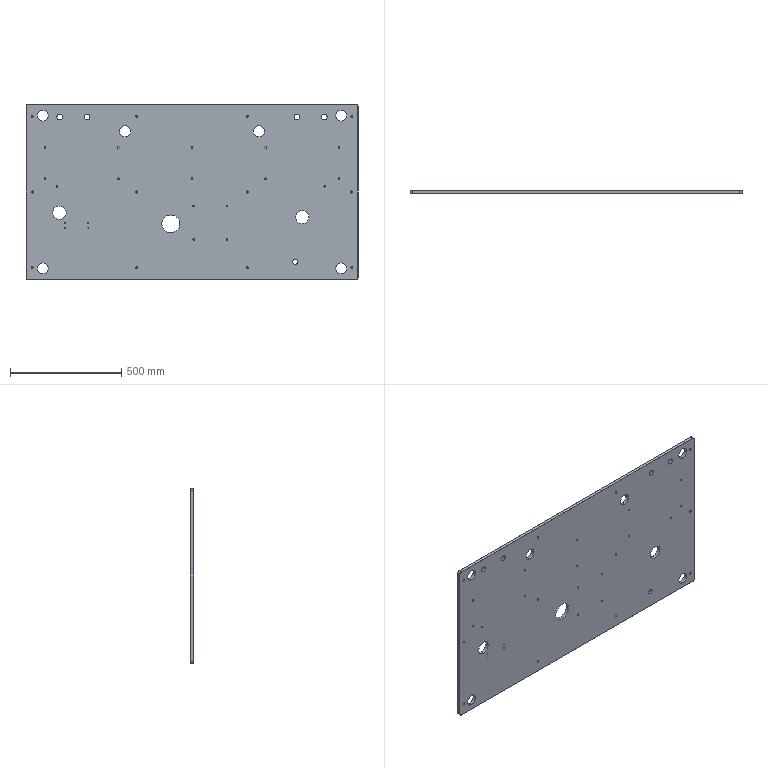Part | STEP file | ND25021-01-JDKM-103-TL | 1 solid | 160 faces | box 1490 x 15 x 786 mm | volume 17159345 mm3 | cylinder 124 | plane 28 | cone 8 | commonest cylinder face diameters 6.8 x28 9 x24 15 x24 50 x12 3.3 x8 25 x8